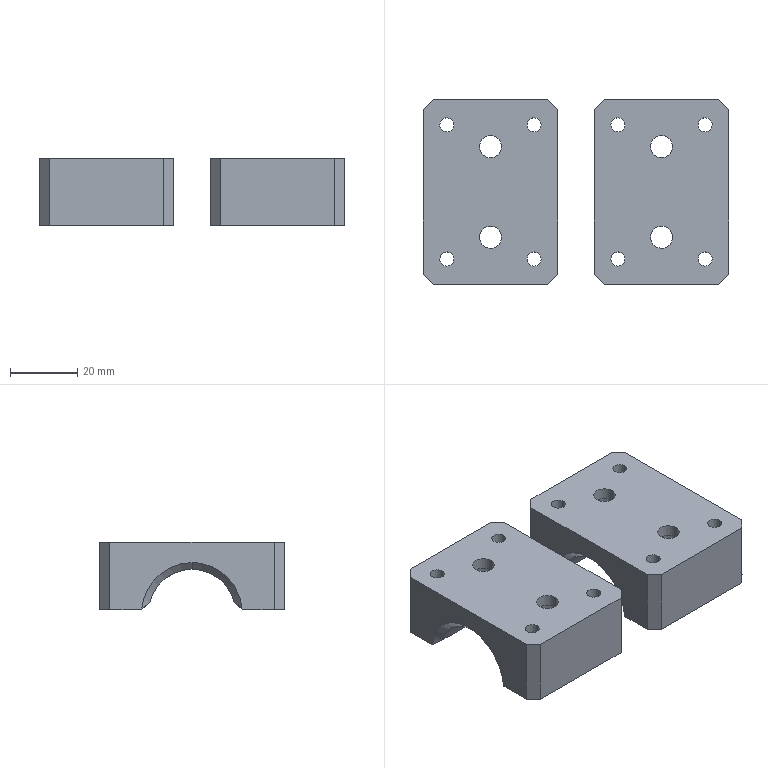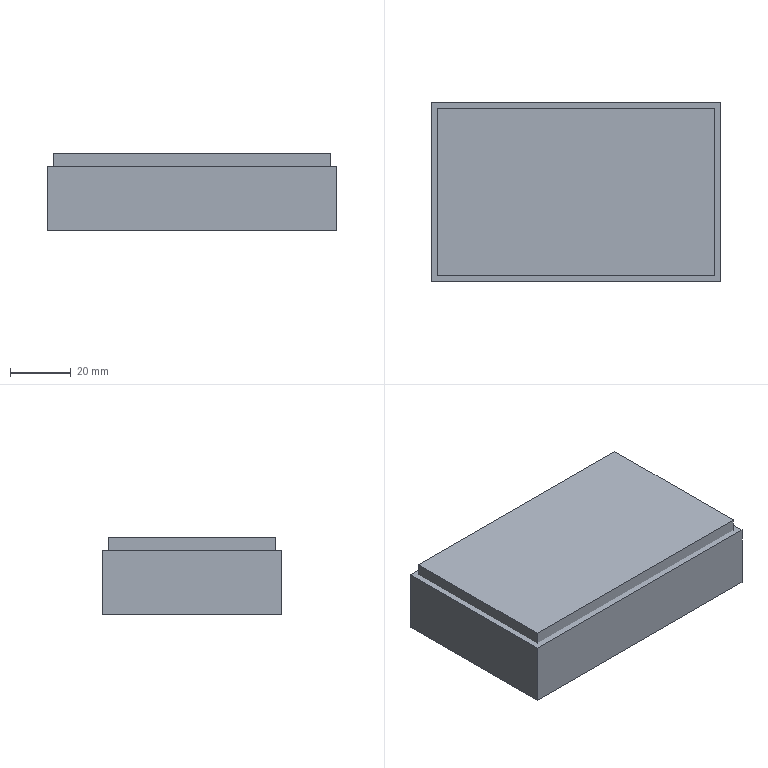CAM job | NX | 3-axis milling, drilling | part box 91 x 55 x 20 mm | stock box 95 x 59 x 25 mm
Tools:
number,name,description,diameter,corner_radius,flute_length,length,flutes
19,D80,Milling Tool-5 Parameters,80.0,0.0,50.0,75.0,2
15,D10,Milling Tool-5 Parameters,10.0,0.0,50.0,75.0,2
1,D6A45,Milling Tool-5 Parameters,6.0,0.0,50.0,75.0,2
4,4.2ZT,Drilling Tool,4.2,0.0,35.0,50.0,2
16,6.6ZT,Drilling Tool,6.6,0.0,35.0,50.0,2
12,D6,Milling Tool-5 Parameters,6.0,0.0,50.0,75.0,2
17,R3,Milling Tool-5 Parameters,6.0,3.0,50.0,75.0,2
14,D10JING,Milling Tool-5 Parameters,10.0,0.0,50.0,75.0,2
Operations:
program,operation,operation_type,tool,method,geometry_group,spindle_rpm,surface_speed,feed_per_tooth,feed_cut,feed_plunge,cut_length_mm,path_length_mm,cut_time_min,machine_time_min
1,FLOOR_WALL_COPY,VolumeBased25DMillingOperation,D80,METHOD,A,6500.0,1633.0,0.1154,1500.0,100.0,191.0,245.0,0.1273,0.1327
1,DRILLING_COPY_1,Operation,D6A45,METHOD,A,5000.0,94.0,0.035,350.0,0.0,62.4,426.998,0.1783,0.2147
1,DRILLING_COPY_COPY,Operation,4.2ZT,METHOD,A,2000.0,20.0,0.045,180.0,0.0,206.095,688.35,1.145,1.193
1,DRILLING_COPY_COPY_COPY,Operation,6.6ZT,METHOD,A,2000.0,20.0,0.045,180.0,0.0,105.931,386.283,0.5885,0.6165
1,ZLEVEL_PROFILE,ZLevelMilling,D10,METHOD,A,9500.0,298.0,0.1474,2800.0,1000.0,8814.004,9067.197,3.209,3.235
1,CAVITY_MILL,CavityMilling,D10,METHOD,A,9500.0,298.0,0.1316,2500.0,700.0,5386.182,6926.016,3.139,3.293
1,ZLEVEL_PROFILE_COPY_1_COPY_COPY_1,ZLevelMilling,D10JING,METHOD,A,9500.0,298.0,0.0632,1200.0,1000.0,443.45,801.101,0.3707,0.4065
1,HOLE_MILLING,CylinderMilling,D6,METHOD,A,9500.0,179.0,0.0737,1400.0,100.0,2231.613,2640.613,1.594,1.635
1,CAVITY_MILL_COPY,CavityMilling,D6,METHOD,A,9500.0,179.0,0.0789,1500.0,700.0,379.015,638.048,0.2659,0.2918
1,FIXED_CONTOUR,SurfaceContour,R3,METHOD,A,9500.0,179.0,0.1579,3000.0,1000.0,44619.204,45304.597,14.925,14.994
1,PLANAR_MILL_COPY_COPY_COPY_COPY_COPY_COPY_1,PlanarMilling,D6A45,METHOD,A,9500.0,179.0,0.0658,1250.0,100.0,460.587,1755.274,0.3685,0.4979
2,FLOOR_WALL_COPY_COPY,VolumeBased25DMillingOperation,D80,METHOD,B,6500.0,1633.0,0.1154,1500.0,100.0,935.0,1909.001,0.6233,0.7207
2,PLANAR_MILL_COPY_COPY_COPY_COPY_COPY_COPY_1_1,PlanarMilling,D6A45,METHOD,B,9500.0,179.0,0.0658,1250.0,100.0,569.157,1645.129,0.4553,0.5629